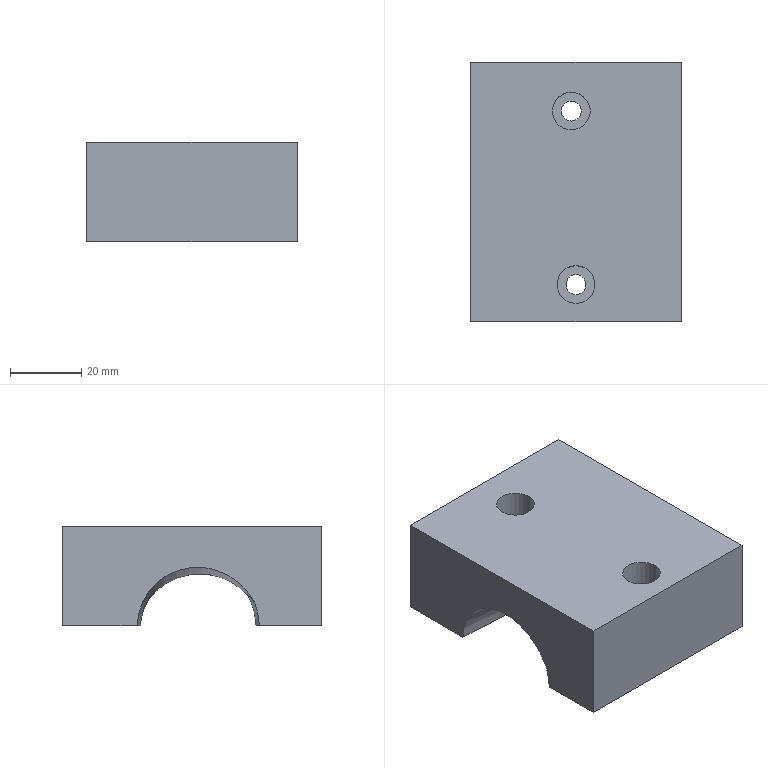NC program | NX | posted with a generic post | part box 59.014 x 72.744 x 27.972 mm
Lines 1 to 1690 of 94199, first 1532 of 1680 lines:
N10 G17 G21 G94 G90
(FLOOR_WALL_COPY_1 , TOOL : D63)
N12 T03 M6
N14 G54
N16 G17 G0 G90 X70.872 Y0. S6500 M3
N18 G43 Z30. H3
N20 Z10.025
N22 G94 G1 Z7.025 F1500.
N24 X67.872
N26 X-67.872
N28 X-70.872
N30 Z10.025
N32 G0 Z30.
N34 X70.872
N36 Z9.05
N38 G1 Z6.05
N40 X67.872
N42 X-67.872
N44 X-70.872
N46 Z9.05
N48 G0 Z30.
N50 X70.872
N52 Z8.075
N54 G1 Z5.075
N56 X67.872
N58 X-67.872
N60 X-70.872
N62 Z8.075
N64 G0 Z30.
N66 X70.872
N68 Z7.1
N70 G1 Z4.1
N72 X67.872
N74 X-67.872
N76 X-70.872
N78 Z7.1
N80 G0 Z30.
N82 X70.872
N84 Z6.125
N86 G1 Z3.125
N88 X67.872
N90 X-67.872
N92 X-70.872
N94 Z6.125
N96 G0 Z30.
N98 X70.872
N100 Z5.15
N102 G1 Z2.15
N104 X67.872
N106 X-67.872
N108 X-70.872
N110 Z5.15
N112 G0 Z30.
N114 X70.872
N116 Z4.175
N118 G1 Z1.175
N120 X67.872
N122 X-67.872
N124 X-70.872
N126 Z4.175
N128 G0 Z30.
N130 X70.872
N132 Z3.2
N134 G1 Z0.2
N136 X67.872
N138 X-67.872
N140 X-70.872
N142 Z3.2
N144 G0 Z30.
(FLOOR_WALL_COPY , TOOL : D63)
N146 X70.872
N148 Z3.
N150 G1 Z0.
N152 X67.872
N154 X-67.872
N156 X-70.872
N158 Z3.
N160 G0 Z30.
N162 M5
(ZLEVEL_PROFILE , TOOL : D10)
N164 T04 M6
N166 G54
N168 G17 G0 G90 X10.244 Y-35.541 S9500 M3
N170 G43 Z30. H4
N172 Z2.351
N174 G94 G1 Z-0.649 F1000.
N176 X12.69 Y-34.597
N178 G3 X13.318 Y-33.819 R1.
N180 G1 X13.332 Y-33.732 F3000.
N182 X14.234 Y-29.123
N184 X14.348 Y-28.585
N186 G3 X15.286 Y-19.404 R55.709
N188 X15.197 Y-18.502 R3.88
N190 G2 X13.462 Y5.443 R84.392
N192 G3 X13.42 Y6.979 R16.351
N194 G2 X13.599 Y29.292 R84.224
N196 X14.545 Y35.573 R362.838
N198 G1 X14.514 Y35.601 Z-1.296
N200 X14.477 Y35.4
N202 X13.767 Y30.791
N204 X13.538 Y29.165
N206 G3 X13.212 Y8.399 R83.745
N208 G1 X13.367 Y6.979
N210 G2 X13.409 Y5.443 R10.635
N212 G1 X13.319 Y3.906
N214 G3 X15.187 Y-18.634 R84.172
N216 G2 X15.254 Y-19.312 R2.871
N218 X14.202 Y-29.091 R56.887
N220 G1 X13.271 Y-33.837
N222 X13.192 Y-33.856 Z-1.939
N224 X14.151 Y-28.974
N226 G3 X15.176 Y-19.101 R54.964
N228 X15.131 Y-18.665 R1.888
N230 G2 X13.335 Y5.389 R83.356
N232 G3 X13.292 Y7.073 R8.768
N234 G2 X12.679 Y20.037 R87.094
N236 X13.595 Y30.023 R85.945
N238 G1 X14.407 Y35.4
N240 X14.453 Y35.633
N242 X14.376 Y35.669 Z-2.577
N244 X14.325 Y35.4
N246 X13.614 Y30.791
N248 X13.503 Y30.023
N250 G3 X13.162 Y7.448 R83.572
N252 G2 X13.221 Y5.23 R11.833
N254 G3 X14.985 Y-18.431 R83.939
N256 G2 X15.081 Y-19.474 R4.204
N258 G1 X15.066 Y-19.906
N260 G2 X14.088 Y-28.822 R52.674
N262 G1 X13.094 Y-33.866
N264 X13.021 Y-33.87 Z-2.893
N266 X12.961 Y-33.873 Z-3.208
N268 X12.981 Y-33.732
N270 X13.937 Y-28.998
N272 G3 X14.969 Y-19.654 R52.682
N274 X14.945 Y-18.706 R10.436
N276 G2 X13.103 Y5.296 R82.541
N278 G3 X13.052 Y7.356 R10.887
N280 G2 X12.975 Y26.95 R84.718
N282 X14.252 Y35.611 R281.865
N284 G1 X14.116 Y35.519 Z-3.831
N286 X13.489 Y31.559
N288 G3 X12.681 Y25.414 R113.024
N290 X12.88 Y7.747 R82.659
N292 G2 X12.963 Y5.443 R12.695
N294 G1 X12.92 Y4.674
N296 G3 X14.798 Y-18.645 R82.137
N298 G2 X14.851 Y-19.161 R2.163
N300 X13.936 Y-28.355 R56.288
N302 G1 X13.76 Y-29.123
N304 X12.982 Y-32.964
N306 X12.817 Y-33.879
N308 X12.738 Y-33.875 Z-4.138
N310 X12.645 Y-33.87 Z-4.444
N312 X13.916 Y-27.587
N314 G3 X14.7 Y-19.181 R54.369
N316 X14.643 Y-18.64 R2.276
N318 G2 X12.613 Y1.602 R82.074
N320 G1 X12.766 Y4.674
N322 X12.804 Y5.243
N324 G3 X12.733 Y7.747 R12.341
N326 G2 X12.89 Y28.486 R80.701
N328 X13.945 Y35.437 R440.926
N330 G1 X13.639 Y35.3 Z-5.043
N332 G2 X13.058 Y30.791 R60.606
N334 G1 X12.611 Y27.718
N336 X12.526 Y26.95
N338 G3 X12.557 Y7.747 R81.878
N340 G2 X12.633 Y5.443 R13.099
N342 G1 X12.577 Y4.674
N344 G3 X14.438 Y-18.464 R80.595
N346 G2 X14.522 Y-19.342 R3.428
N348 G1 X14.503 Y-19.906
N350 G2 X13.428 Y-29.123 R47.968
N352 G1 X13.268 Y-29.891
N354 X12.462 Y-33.858
N356 X12.356 Y-33.85 Z-5.334
N358 X12.255 Y-33.843 Z-5.624
N360 X12.436 Y-32.964
N362 X13.307 Y-28.768
N364 G3 X14.348 Y-18.823 R49.962
N366 G2 X12.436 Y5.443 R79.079
N368 G3 X12.379 Y7.747 R12.329
N370 G2 X12.653 Y29.255 R79.978
N372 G1 X12.804 Y30.213
N374 G3 X13.315 Y35.262 R56.984
N376 G1 X13.156 Y35.269 Z-5.908
N378 X12.997 Y35.276 Z-6.193
N380 G2 X12.572 Y30.023 R134.005
N382 G3 X12.175 Y7.747 R80.176
N384 G2 X12.216 Y5.443 R10.851
N386 G3 X13.867 Y-17.601 R78.874
N388 G1 X14.077 Y-18.541
N390 G2 X14.133 Y-19.113 R2.338
N392 G1 X14.112 Y-19.906
N394 G2 X13.192 Y-28.355 R48.034
N396 G1 X13.019 Y-29.123
N398 X12.034 Y-33.824
N400 X11.916 Y-33.817 Z-6.473
N402 X11.785 Y-33.81 Z-6.754
N404 X12.804 Y-29.067
N406 G3 X13.907 Y-18.725 R47.797
N408 G2 X11.831 Y3.138 R79.078
N410 G1 X11.992 Y5.443
N412 G3 X11.967 Y7.747 R11.595
N414 G2 X12.241 Y29.225 R78.57
N416 G3 X12.348 Y30.277 R10.864
N418 G1 X12.415 Y31.559
N420 X12.683 Y35.289
N422 X12.529 Y35.295 Z-7.026
N424 X12.378 Y35.302 Z-7.298
N426 X11.899 Y28.486
N428 G3 X11.3 Y12.356 R79.402
N430 G2 X11.737 Y6.445 R297.99
N432 X11.712 Y4.878 R9.86
N434 G1 X11.619 Y3.906
N436 G3 X13.688 Y-18.749 R78.587
N438 G2 X12.804 Y-27.88 R49.81
N440 G3 X11.519 Y-33.792 R606.821
N442 G1 X11.381 Y-33.782 Z-7.56
N444 X11.244 Y-33.772 Z-7.821
N446 X11.41 Y-32.964
N448 X12.379 Y-28.643
N450 G3 X13.352 Y-21.174 R41.302
N452 G1 X13.447 Y-18.69
N454 G2 X11.377 Y3.906 R77.127
N456 G1 X11.422 Y4.436
N458 G3 X11.43 Y5.461 R6.681
N460 G2 X10.943 Y14.881 R273.148
N462 X11.457 Y26.95 R78.516
N464 G1 X12.089 Y35.314
N466 X11.944 Y35.329 Z-8.073
N468 X11.782 Y35.346 Z-8.324
N470 X11.054 Y26.182
N472 G3 X10.725 Y10.051 R124.668
N474 G1 X10.763 Y9.283
N476 X11.129 Y3.906
N478 G3 X10.98 Y-1.471 R74.898
N480 X12.948 Y-17.601 R78.619
N482 G1 X13.123 Y-18.369
N484 X13.163 Y-18.722
N486 X13.146 Y-19.138
N488 G2 X12.165 Y-28.355 R43.893
N490 G1 X10.936 Y-33.75
N492 X10.797 Y-33.74 Z-8.568
N494 X10.64 Y-33.728 Z-8.811
N496 X12.032 Y-27.679
N498 G3 X12.891 Y-18.369 R46.52
N500 G2 X10.715 Y-1.471 R76.841
N502 X10.813 Y3.138 R82.834
N504 X10.669 Y26.182 R122.396
N506 G1 X11.485 Y35.381
N508 X11.343 Y35.398 Z-9.045
N510 X11.183 Y35.416 Z-9.28
N512 X10.273 Y26.182
N514 X10.091 Y23.878
N516 G3 X10.495 Y2.37 R109.189
N518 X10.461 Y0.272 R151.602
N520 X12.548 Y-17.983 R74.643
N522 G1 X12.604 Y-18.369
N524 X12.588 Y-19.138
N526 G2 X11.55 Y-28.419 R39.567
N528 G1 X10.316 Y-33.701
N530 X10.158 Y-33.687 Z-9.505
N532 X9.985 Y-33.671 Z-9.73
N534 X11.245 Y-28.485
N536 G3 X12.228 Y-21.088 R35.213
N538 G1 X12.308 Y-18.011
N540 G2 X10.189 Y0.408 R73.141
N542 G3 X10.105 Y1.844 R10.172
N544 G2 X9.604 Y22.746 R99.677
N546 G1 X9.883 Y26.182
N548 X10.858 Y35.453
N550 X10.708 Y35.47 Z-9.946
N552 X10.545 Y35.489 Z-10.162
N554 X9.422 Y25.517
N556 G3 X9.477 Y3.341 R96.947
N558 X9.896 Y0.066 R161.578
N560 X11.963 Y-17.601 R73.39
N562 G2 X11.996 Y-19.138 R6.001
N564 X10.91 Y-28.55 R37.741
N566 G1 X9.659 Y-33.641
N568 X9.491 Y-33.624 Z-10.368
N570 X9.311 Y-33.605 Z-10.574
N572 G3 X11.134 Y-26.051 R120.535
N574 X11.69 Y-17.601 R44.58
N576 G2 X9.642 Y-1.548 R74.685
N578 G3 X9.57 Y-0.692 R6.581
N580 G1 X9.226 Y1.602
N582 G2 X8.844 Y23.878 R87.033
N584 G1 X9.083 Y26.182
N586 X10.21 Y35.526
N588 X10.053 Y35.544 Z-10.77
N590 X9.883 Y35.563 Z-10.967
N592 X8.605 Y25.669
N594 G3 X7.81 Y11.588 R97.875
N596 X9.369 Y-2.239 R99.053
N598 X11.367 Y-17.248 R75.126
N600 G2 X10.489 Y-27.731 R40.2
N602 G1 X8.978 Y-33.569
N604 X8.812 Y-33.552 Z-11.153
N606 X8.618 Y-33.531 Z-11.339
N608 X10.192 Y-27.587
N610 X10.37 Y-26.819
N612 G3 X11.031 Y-16.833 R40.131
N614 G2 X9.168 Y-3.775 R73.819
N616 X8.033 Y3.138 R985.26
N618 X7.859 Y23.11 R75.535
N620 X9.553 Y35.6 R1001.089
N622 G1 X9.386 Y35.618 Z-11.515
N624 X9.221 Y35.637 Z-11.691
N626 X7.713 Y25.414
N628 X7.243 Y21.624
N630 G3 X7.41 Y3.969 R66.674
N632 X8.945 Y-4.75 R138.157
N634 X10.616 Y-16.065 R80.897
N636 G2 X9.717 Y-28.269 R35.231
N638 G1 X8.271 Y-33.492
N640 X8.094 Y-33.472 Z-11.857
N642 X7.911 Y-33.45 Z-12.022
N644 X8.051 Y-32.964
N646 X9.717 Y-26.986
N648 G3 X10.21 Y-15.297 R35.008
N650 G2 X8.783 Y-6.079 R90.765
N652 G1 X7.545 Y0.066
N654 X7.265 Y1.537
N656 G2 X6.648 Y20.47 R61.369
N658 G1 X7.067 Y23.878
N660 X8.901 Y35.672
N662 X8.729 Y35.692 Z-12.177
N664 X8.566 Y35.71 Z-12.332
N666 X6.502 Y23.11
N668 X6.143 Y20.353
N670 G3 X5.885 Y6.979 R60.76
N672 X8.557 Y-6.848 R140.299
N674 X9.949 Y-15.297 R169.214
N676 G2 X9.44 Y-26.819 R36.947
N678 G1 X9.249 Y-27.587
N680 X7.564 Y-33.408
N682 X7.391 Y-33.385 Z-12.477
N684 X7.221 Y-33.362 Z-12.622
N686 X7.401 Y-32.789
N688 X8.945 Y-27.627
N690 X9.141 Y-26.819
N692 G3 X9.42 Y-13.761 R35.75
N694 G1 X9.272 Y-12.993
N696 X9.144 Y-12.224
N698 G3 X6.773 Y-1.013 R134.514
N700 G2 X5.584 Y19.772 R54.025
N702 G1 X6.043 Y23.11
N704 X8.25 Y35.746
N706 X8.091 Y35.765 Z-12.756
N708 X7.934 Y35.784 Z-12.889
N710 X5.599 Y23.11
N712 X5.259 Y20.805
N714 X4.933 Y18.628
N716 G3 X5.416 Y2.983 R43.75
N718 G1 X6.204 Y-0.702
N720 G2 X9.227 Y-14.529 R118.409
N722 X8.854 Y-26.819 R34.94
N724 G1 X8.648 Y-27.587
N726 X6.885 Y-33.313
N728 X6.728 Y-33.289 Z-13.012
N730 X6.566 Y-33.264 Z-13.134
N732 X8.365 Y-27.587
N734 X8.568 Y-26.819
N736 G3 X8.945 Y-14.695 R32.979
N738 X6.132 Y-2.239 R98.202
N740 G2 X3.925 Y9.283 R55.566
N742 X4.729 Y20.551 R50.892
N744 G1 X5.085 Y22.483
N746 X5.178 Y23.11
N748 X7.638 Y35.821
N750 X7.501 Y35.838 Z-13.246
N752 X7.363 Y35.855 Z-13.358
N754 X4.313 Y20.873
N756 X4.151 Y20.037
N758 G3 X3.896 Y4.674 R42.458
N760 G1 X4.234 Y3.138
N762 X7.18 Y-7.665
N764 G2 X8.969 Y-17.421 R58.43
N766 X7.859 Y-28.355 R28.007
N768 G1 X6.252 Y-33.209
N770 X6.108 Y-33.184 Z-13.458
N772 X5.965 Y-33.159 Z-13.558
N774 X7.84 Y-27.587
N776 X8.061 Y-26.819
N778 G3 X8.463 Y-15.297 R29.811
N780 X5.469 Y-3.007 R77.185
N782 G1 X4.962 Y-1.471
N784 G2 X2.755 Y8.515 R55.165
N786 X3.459 Y18.844 R39.058
N788 G1 X3.858 Y20.805
N790 X6.629 Y33.506
N792 X7.097 Y35.891
N794 G3 X6.773 Y36.837 R1.
N796 G1 X4.848 Y38.516
N798 Z-10.558
N800 G0 Z30.
N802 X-7.808 Y37.382
N804 Z2.351
N806 G1 Z-0.649 F1000.
N808 X-9.983 Y35.98
N810 G3 X-10.44 Y35.091 R1.
N812 G2 X-10.193 Y29.255 R446.101 F3000.
N814 G1 X-9.511 Y16.964
N816 X-9.407 Y14.793
N818 G2 X-9.866 Y-3.186 R122.787
N820 G1 X-10.762 Y-12.224
N822 G3 X-11.187 Y-19.963 R97.835
N824 X-10.376 Y-29.019 R43.623
N826 G1 X-9.436 Y-33.815
N828 X-9.387 Y-33.83 Z-1.296
N830 X-9.544 Y-32.964
N832 X-10.302 Y-29.123
N834 X-10.353 Y-28.92
N836 G2 X-11.028 Y-23.746 R39.014
N838 G1 X-11.057 Y-22.978
N840 X-11.124 Y-22.21
N842 G2 X-11.124 Y-18.453 R110.474
N844 G3 X-11.013 Y-16.065 R46.666
N846 G2 X-10.359 Y-8.611 R202.692
N848 G3 X-9.645 Y-1.471 R585.412
N850 X-9.205 Y8.515 R113.819
N852 X-9.378 Y15.428 R152.84
N854 X-9.987 Y26.182 R461.108
N856 G1 X-10.37 Y34.631
N858 X-10.396 Y35.144
N860 X-10.335 Y35.186 Z-1.939
N862 X-10.3 Y34.631
N864 X-9.981 Y27.718
N866 X-9.938 Y26.95
N868 X-9.35 Y16.964
N870 X-9.244 Y14.66
N872 G2 X-9.699 Y-3.007 R118.11
N874 G1 X-9.847 Y-4.543
N876 X-10.49 Y-10.688
N878 G3 X-11.07 Y-20.674 R99.491
N880 X-10.53 Y-27.587 R47.233
N882 G1 X-10.393 Y-28.355
N884 X-9.314 Y-33.847
N886 X-9.208 Y-33.857 Z-2.577
N888 X-10.256 Y-28.514
N890 G2 X-10.905 Y-23.146 R36.873
N892 X-10.734 Y-14.529 R64.491
N894 X-9.742 Y-4.543 R359.94
N896 G3 X-9.043 Y4.674 R146.008
N898 X-9.076 Y13.327 R130.573
N900 X-9.504 Y21.563 R276.789
N902 G2 X-10.24 Y35.195 R530.755
N904 G1 X-10.185 Y35.199 Z-2.893
N906 X-10.139 Y35.203 Z-3.208
N908 G3 X-9.666 Y26.182 R1124.487
N910 G1 X-9.516 Y23.878
N912 X-9.465 Y23.11
N914 G2 X-9.04 Y16.139 R568.997
N916 X-8.909 Y3.906 R139.195
N918 X-9.842 Y-6.848 R174.936
N920 G3 X-10.675 Y-15.363 R223.861
N922 X-10.765 Y-23.746 R62.101
N924 X-10.029 Y-29.123 R37.612
N926 G1 X-9.867 Y-29.891
N928 X-9.086 Y-33.863
N930 X-9.008 Y-33.864 Z-3.52
N932 X-8.934 Y-33.866 Z-3.831
N934 X-9.889 Y-29.123
N936 X-10.051 Y-28.355
N938 G2 X-10.662 Y-17.601 R45.697
N940 X-9.935 Y-9.152 R127.722
N942 G3 X-9.053 Y-0.702 R291.588
N944 X-8.667 Y11.588 R104.753
N946 G1 X-8.99 Y18.501
N948 G2 X-9.996 Y35.215 R769.386
N950 G1 X-9.91 Y35.221 Z-4.138
N952 X-9.822 Y35.227 Z-4.444
N954 G3 X-9.186 Y23.878 R640.786
N956 G1 X-9.056 Y22.341
N958 X-8.996 Y21.573
N960 X-8.966 Y20.805
N962 G2 X-8.516 Y13.124 R231.159
N964 X-8.986 Y-2.239 R105.26
N966 X-9.932 Y-10.688 R781.442
N968 G3 X-10.565 Y-18.951 R114.064
N970 X-9.756 Y-29.016 R42.1
N972 G1 X-8.798 Y-33.732
N974 X-8.777 Y-33.867
N976 X-8.678 Y-33.862 Z-4.744
N978 X-8.583 Y-33.857 Z-5.043
N980 X-9.581 Y-29.031
N982 G2 X-10.388 Y-19.222 R41.455
N984 X-9.75 Y-10.879 R106.308
N986 G1 X-8.925 Y-3.775
N988 X-8.764 Y-2.239
N990 G3 X-8.225 Y11.588 R99.983
N992 X-8.731 Y20.805 R225.203
N994 G2 X-9.644 Y35.24 R426.911
N996 G1 X-9.553 Y35.246 Z-5.334
N998 X-9.447 Y35.252 Z-5.624
N1000 G3 X-8.809 Y24.739 R449.887
N1002 G1 X-8.665 Y23.11
N1004 X-8.268 Y17.548
N1006 G2 X-7.92 Y8.324 R136.877
N1008 X-8.282 Y0.222 R83.479
N1010 G1 X-8.512 Y-2.239
N1012 X-8.579 Y-3.007
N1014 X-8.674 Y-3.775
N1016 X-8.776 Y-4.543
N1018 X-9.684 Y-12.224
N1020 X-9.894 Y-14.461
N1022 G3 X-10.21 Y-20.861 R72.663
N1024 X-9.41 Y-28.89 R38.624
N1026 G1 X-8.385 Y-33.846
N1028 X-8.262 Y-33.837 Z-5.908
N1030 X-8.15 Y-33.829 Z-6.193
N1032 X-9.305 Y-28.355
N1034 G2 X-9.958 Y-18.369 R40.916
N1036 X-8.891 Y-7.616 R141.923
N1038 G3 X-8.306 Y-3.007 R212.591
N1040 G1 X-8.238 Y-2.239
N1042 X-8.065 Y-0.702
N1044 X-7.914 Y1.064
N1046 G3 X-7.681 Y12.195 R86.708
N1048 G1 X-7.755 Y13.892
N1050 G3 X-8.353 Y22.341 R271.693
N1052 G2 X-9.241 Y35.264 R406.061
N1054 G1 X-9.121 Y35.271 Z-6.473
N1056 X-9.003 Y35.278 Z-6.754
N1058 G3 X-8.001 Y21.573 R369.34
N1060 G1 X-7.933 Y20.805
N1062 X-7.596 Y16.32
N1064 G2 X-7.43 Y3.138 R105.532
N1066 G1 X-7.759 Y-0.702
N1068 G2 X-8.908 Y-9.92 R320.186
N1070 G3 X-9.756 Y-19.405 R101.404
N1072 X-8.947 Y-28.933 R37.787
N1074 G1 X-7.9 Y-33.812
N1076 X-7.77 Y-33.804 Z-7.026
N1078 X-7.638 Y-33.796 Z-7.298
N1080 X-7.796 Y-32.964
N1082 X-8.686 Y-28.978
N1084 G2 X-9.531 Y-20.649 R35.322
N1086 X-8.856 Y-11.678 R78.251
N1088 G1 X-7.595 Y-2.239
N1090 X-7.52 Y-1.471
N1092 X-7.423 Y-0.702
N1094 G3 X-7.107 Y13.892 R86.944
N1096 X-8.037 Y25.194 R275.313
N1098 G1 X-8.421 Y30.023
N1100 G3 X-8.753 Y35.293 R145.709
N1102 G1 X-8.623 Y35.302 Z-7.56
N1104 X-8.477 Y35.311 Z-7.821
N1106 G3 X-7.368 Y21.573 R313.598
N1108 G2 X-6.633 Y11.438 R148.06
N1110 X-7.282 Y-2.359 R81.406
N1112 X-8.475 Y-11.072 R1051.255
N1114 G3 X-9.215 Y-18.439 R92.262
N1116 X-8.809 Y-27.086 R40.563
N1118 X-7.357 Y-33.775 R1700.526
N1120 G1 X-7.208 Y-33.763 Z-8.073
N1122 X-7.057 Y-33.751 Z-8.324
N1124 X-8.105 Y-29.123
N1126 G2 X-8.872 Y-24.514 R35.129
N1128 X-8.672 Y-15.297 R47.716
N1130 X-7.235 Y-4.693 R225.714
N1132 G3 X-6.326 Y13.195 R83.374
N1134 X-7.055 Y21.977 R169.123
N1136 G2 X-8.205 Y35.329 R290.272
N1138 G1 X-8.077 Y35.338 Z-8.568
N1140 X-7.925 Y35.348 Z-8.811
N1142 X-7.25 Y26.95
N1144 G2 X-6.015 Y14.66 R310.631
N1146 X-6.631 Y-3.007 R77.1
N1148 X-7.796 Y-10.719 R2179.035
N1150 G3 X-8.69 Y-19.311 R90.208
N1152 X-7.85 Y-29.019 R34.378
N1154 G1 X-6.755 Y-33.726
N1156 X-6.598 Y-33.712 Z-9.045
N1158 X-6.438 Y-33.698 Z-9.28
N1160 X-7.697 Y-28.355
N1162 G2 X-8.434 Y-20.865 R30.899
N1164 X-7.716 Y-12.459 R68.938
N1166 G1 X-7.341 Y-9.92
N1168 X-6.351 Y-3.775
N1170 X-6.125 Y-2.239
N1172 G3 X-5.388 Y11.588 R76.769
N1174 X-6.409 Y22.689 R193.116
N1176 G2 X-7.62 Y35.37 R250.441
N1178 G1 X-7.489 Y35.38 Z-9.505
N1180 X-7.326 Y35.391 Z-9.73
N1182 X-7.266 Y34.631
N1184 X-6.548 Y26.95
N1186 X-5.71 Y19.967
N1188 G2 X-5.135 Y14.438 R175.423
N1190 X-5.654 Y-1.793 R67.999
N1192 X-6.983 Y-9.92 R396.157
N1194 G3 X-8.094 Y-19.138 R82.702
N1196 X-7.212 Y-29.123 R32.402
N1198 G1 X-7.022 Y-29.891
N1200 X-6.104 Y-33.665
N1202 X-5.962 Y-33.651 Z-9.946
N1204 X-5.784 Y-33.634 Z-10.162
N1206 X-7.266 Y-27.587
N1208 G2 X-7.731 Y-18.369 R33.33
N1210 X-6.357 Y-8.384 R89.029
N1212 G3 X-4.501 Y4.674 R113.083
N1214 X-5.192 Y19.269 R81.307
N1216 G2 X-7.01 Y35.415 R295.073
N1218 G1 X-6.862 Y35.427 Z-10.368
N1220 X-6.694 Y35.44 Z-10.574
N1222 G3 X-4.561 Y17.733 R329.111
N1224 G2 X-4.142 Y3.138 R68.234
N1226 X-5.972 Y-8.384 R129.415
N1228 G3 X-7.431 Y-18.369 R89.492
N1230 X-6.493 Y-29.503 R31.685
N1232 G1 X-5.432 Y-33.602
N1234 X-5.263 Y-33.586 Z-10.77
N1236 X-5.085 Y-33.571 Z-10.967
N1238 X-6.277 Y-29.034
N1240 G2 X-7.083 Y-17.889 R30.423
N1242 X-5.126 Y-6.079 R115.645
N1244 G3 X-3.484 Y5.443 R84.483
N1246 X-4.3 Y19.269 R73.
N1248 G2 X-6.378 Y35.465 R249.012
N1250 G1 X-6.222 Y35.478 Z-11.153
N1252 X-6.051 Y35.493 Z-11.339
N1254 G3 X-3.966 Y19.998 R236.49
N1256 G2 X-2.878 Y7.747 R78.74
N1258 X-4.517 Y-5.114 R69.218
N1260 G3 X-6.551 Y-16.065 R150.783
N1262 X-6.482 Y-26.819 R34.194
N1264 G1 X-6.31 Y-27.587
N1266 X-4.73 Y-33.535
N1268 X-4.557 Y-33.516 Z-11.515
N1270 X-4.378 Y-33.496 Z-11.691
N1272 X-5.81 Y-28.355
N1274 G2 X-6.42 Y-17.601 R29.376
N1276 X-4.126 Y-5.311 R120.054
N1278 G3 X-2.347 Y7.747 R63.655
N1280 X-3.511 Y20.037 R70.245
N1282 G2 X-5.74 Y35.52 R236.179
N1284 G1 X-5.575 Y35.535 Z-11.857
N1286 X-5.408 Y35.551 Z-12.022
N1288 G3 X-2.775 Y18.501 R235.49
N1290 G2 X-3.406 Y-4.04 R52.249
N1292 G3 X-5.902 Y-16.065 R165.767
N1294 X-5.854 Y-26.819 R31.71
N1296 G1 X-5.721 Y-27.442
N1298 X-4.029 Y-33.455
N1300 X-3.856 Y-33.432 Z-12.177
N1302 X-3.679 Y-33.409 Z-12.332
N1304 X-4.996 Y-28.933
N1306 G2 X-5.873 Y-18.367 R26.25
N1308 X-3.632 Y-6.848 R82.071
N1310 G3 X-1.338 Y5.443 R77.728
N1312 X-2.278 Y18.501 R51.939
N1314 G2 X-5.095 Y35.581 R216.921
N1316 G1 X-4.94 Y35.597 Z-12.477
N1318 X-4.784 Y35.612 Z-12.622
N1320 G3 X-1.929 Y19.269 R178.983
N1322 G2 X-1.396 Y0.834 R45.853
N1324 G1 X-1.712 Y-0.702
N1326 X-4.177 Y-10.65
N1328 G3 X-5.713 Y-20.154 R53.751
N1330 X-4.766 Y-28.637 R23.626
N1332 G1 X-3.341 Y-33.363
N1334 X-3.173 Y-33.338 Z-12.756
N1336 X-3.002 Y-33.312 Z-12.889
N1338 X-4.361 Y-28.986
N1340 G2 X-5.303 Y-18.596 R24.564
N1342 X-3.026 Y-7.616 R69.397
N1344 G3 X-0.48 Y3.138 R99.8
N1346 X-1.432 Y19.269 R45.088
N1348 G2 X-4.48 Y35.644 R160.733
N1350 G1 X-4.337 Y35.66 Z-13.012
N1352 X-4.198 Y35.675 Z-13.134
N1354 G3 X-0.948 Y19.269 R151.009
N1356 G1 X-0.303 Y16.258
N1358 G2 X-0.899 Y-1.387 R36.391
N1360 G3 X-3.869 Y-12.224 R491.006
N1362 X-5.2 Y-21.845 R40.823
N1364 X-4.228 Y-28.452 R20.407
N1366 G1 X-2.685 Y-33.262
N1368 X-2.535 Y-33.235 Z-13.246
N1370 X-2.381 Y-33.207 Z-13.358
N1372 X-2.634 Y-32.471
N1374 X-3.966 Y-28.388
N1376 G2 X-4.938 Y-21.093 R20.243
N1378 X-3.276 Y-11.155 R43.739
N1380 G1 X-0.158 Y-0.357
N1382 G3 X0.406 Y15.18 R32.067
N1384 G1 X-0.459 Y19.269
N1386 G2 X-3.918 Y35.708 R132.758
N1388 G1 X-3.789 Y35.723 Z-13.458
N1390 X-3.659 Y35.739 Z-13.558
N1392 G3 X-0.171 Y20.037 R108.953
N1394 G2 X1.717 Y7.747 R44.161
N1396 X-0.847 Y-4.274 R46.086
N1398 G3 X-4.385 Y-17.601 R81.85
N1400 X-3.406 Y-29.324 R23.181
N1402 G1 X-3.21 Y-29.891
N1404 X-2.097 Y-33.152
N1406 X-1.971 Y-33.128 Z-13.648
N1408 X-1.835 Y-33.101 Z-13.739
N1410 X-3.719 Y-27.587
N1412 X-3.935 Y-26.819
N1414 G2 X-3.887 Y-16.065 R25.126
N1416 X-0.049 Y-3.033 R99.301
N1418 G3 X2.299 Y7.367 R40.248
N1420 X4.539 Y-1.471 R45.918
N1422 G2 X7.82 Y-12.993 R89.022
N1424 X8.182 Y-25.283 R32.816
N1426 X5.693 Y-33.106 R59.891
N1428 G1 X5.555 Y-33.077 Z-13.826
N1430 X5.414 Y-33.047 Z-13.914
N1432 G3 X7.95 Y-25.283 R51.28
N1434 X7.84 Y-14.507 R30.262
N1436 X4.313 Y-2.097 R73.482
N1438 G1 X4.068 Y-1.471
N1440 X2.546 Y3.138
N1442 X2.394 Y3.701
N1444 G2 X-0.693 Y-6.079 R83.994
N1446 G3 X-4.102 Y-18.995 R57.289
N1448 X-3.153 Y-28.569 R20.239
N1450 G1 X-1.862 Y-32.234
N1452 X-1.545 Y-33.042
N1454 X-1.398 Y-33.012 Z-14.001
N1456 X-1.252 Y-32.982 Z-14.088
N1458 X-2.71 Y-29.123
N1460 G2 X-3.953 Y-19.906 R19.59
N1462 X-1.177 Y-8.384 R47.734
N1464 G1 X2.453 Y1.4
N1466 X2.77 Y0.732
N1468 X3.826 Y-2.239
N1470 X4.163 Y-3.007
N1472 G2 X7.838 Y-16.065 R60.096
N1474 X7.361 Y-26.819 R26.457
N1476 G1 X7.122 Y-27.587
N1478 X5.134 Y-32.988
N1480 X4.99 Y-32.951 Z-14.176
N1482 X4.835 Y-32.911 Z-14.263
N1484 G3 X7.485 Y-25.283 R50.071
N1486 X6.993 Y-12.993 R29.609
N1488 X2.521 Y-0.367 R71.88
N1490 X-2.122 Y-12.224 R115.606
N1492 X-3.791 Y-22.613 R32.458
N1494 X-2.647 Y-28.611 R16.585
N1496 G1 X-1.09 Y-32.582
N1498 X-0.946 Y-32.91
N1500 X-0.794 Y-32.872 Z-14.35
N1502 X-0.631 Y-32.831 Z-14.437
N1504 X-2.634 Y-27.854
N1506 G2 X-3.158 Y-17.601 R20.047
N1508 X2.514 Y-1.979 R57.99
N1510 X7.377 Y-16.471 R47.314
N1512 X6.629 Y-27.529 R24.403
N1514 G1 X4.529 Y-32.829
N1516 X4.374 Y-32.785 Z-14.526
N1518 X4.201 Y-32.736 Z-14.615
N1520 X4.313 Y-32.498
N1522 X6.317 Y-27.587
N1524 G3 X7.297 Y-18.079 R22.244
N1526 X2.503 Y-3.347 R38.847
N1528 X-2.882 Y-17.601 R48.23
N1530 X-2.634 Y-27.012 R20.112
N1532 G1 X-2.439 Y-27.587
N1534 X-0.306 Y-32.748
N1536 X-0.138 Y-32.693 Z-14.702
N1538 X0.039 Y-32.636 Z-14.789
N1540 X-1.525 Y-29.123
N1542 G2 X-2.848 Y-19.138 R17.308
N1544 X2.494 Y-4.586 R40.044
N1546 X6.221 Y-13.761 R31.888
N1548 G1 X6.514 Y-15.013
N1550 G2 X6.708 Y-25.283 R24.564
N1552 X3.848 Y-32.629 R38.735
N1554 G1 X3.665 Y-32.569 Z-14.877
N1556 X3.483 Y-32.509 Z-14.966
N1558 G3 X6.707 Y-23.746 R28.391
N1560 X2.501 Y-5.839 R28.375
N1562 X-2.664 Y-19.906 R33.507
N1564 X-1.196 Y-29.123 R16.317
N1566 G1 X0.403 Y-32.514
N1568 X0.593 Y-32.435 Z-15.053
N1570 X0.786 Y-32.354 Z-15.14
N1572 X0.454 Y-31.762
N1574 X-0.834 Y-29.123
N1576 X-1.09 Y-28.58
N1578 G2 X-2.486 Y-21.442 R14.637
N1580 X2.494 Y-6.998 R28.651
N1582 X6.42 Y-23.746 R25.722
N1584 X3.096 Y-32.348 R24.995
N1586 G1 X2.891 Y-32.256 Z-15.229
N1588 X2.684 Y-32.163 Z-15.317
N1590 G3 X5.857 Y-25.147 R26.476
N1592 X2.479 Y-8.051 R23.367
N1594 X-2.187 Y-21.497 R26.173
N1596 X-0.921 Y-28.117 R13.751
N1598 G1 X-0.452 Y-29.123
N1600 X1.196 Y-32.175
N1602 X1.19 Y-31.873 Z-15.376
N1604 X1.187 Y-31.569 Z-15.435
N1606 X1.196 Y-31.258 Z-15.493
N1608 X0.454 Y-30.063
N1610 G2 X-1.902 Y-22.21 R14.837
N1612 X2.471 Y-9.107 R23.636
N1614 X5.815 Y-23.746 R22.089
N1616 X2.265 Y-31.909 R20.488
N1618 G1 X1.998 Y-32.35
N1620 X1.93 Y-32.458
N1622 X1.606 Y-31.916
N1624 X1.196 Y-31.258
N1626 G2 X1.164 Y-30.258 R1.
N1628 G1 X1.923 Y-26.384
N1630 Z-12.493
N1632 G0 Z30.
N1634 X2.658 Y-21.56
N1636 Z-12.671
N1638 G1 Z-15.671 F1000.
N1640 X5.119 Y-19.677
N1642 G3 X5.503 Y-18.754 R1.
N1644 G1 X5.453 Y-18.369 F3000.
N1646 G3 X2.455 Y-10.191 R19.567
N1648 X-1.497 Y-23.746 R20.774
N1650 X1.923 Y-31.464 R16.111
N1652 X5.553 Y-19.138 R16.316
N1654 G1 X5.503 Y-18.754
N1656 X5.337 Y-18.774 Z-15.76
N1658 X5.155 Y-18.796 Z-15.849
N1660 G2 X5.223 Y-19.46 R17.813
N1662 G1 X5.261 Y-19.906
N1664 G2 X1.922 Y-30.575 R14.357
N1666 X-1.16 Y-23.746 R14.056
N1668 X2.429 Y-11.275 R18.829
N1670 X5.155 Y-18.796 R17.813
N1672 G1 X4.964 Y-18.822 Z-15.939
N1674 X4.771 Y-18.848 Z-16.029
N1676 G3 X2.398 Y-12.378 R16.077
N1678 X-0.782 Y-23.746 R16.956
N1680 X1.92 Y-29.671 R11.576
N1682 X4.936 Y-20.674 R12.498
N1684 G1 X4.88 Y-19.906
N1686 G3 X4.771 Y-18.848 R16.077
N1688 G1 X4.566 Y-18.881 Z-16.118
N1690 X4.37 Y-18.912 Z-16.207
N1692 G2 X4.554 Y-21.442 R15.052
N1694 G1 X4.546 Y-22.21
N1696 G2 X1.919 Y-28.783 R10.392
N1698 X-0.425 Y-23.451 R8.655
N1700 X2.371 Y-13.458 R15.391
N1702 X4.37 Y-18.912 R15.052
N1704 G1 X4.153 Y-18.95 Z-16.295
N1706 X3.938 Y-18.989 Z-16.383
N1708 G3 X2.34 Y-14.586 R13.702
N1710 X0.164 Y-24.454 R13.225
N1712 X1.919 Y-27.904 R6.641
N1714 X4.144 Y-22.21 R8.825
N1716 G1 X4.15 Y-21.442
N1718 G3 X3.938 Y-18.989 R13.702
N1720 G1 X3.942 Y-19.344 Z-16.405
N1722 X3.931 Y-19.698 Z-16.428
N1724 X3.91 Y-20.053 Z-16.45
N1726 X3.888 Y-20.408 Z-16.472
N1728 X3.86 Y-20.763 Z-16.494
N1730 X3.811 Y-21.117 Z-16.517
N1732 X3.748 Y-21.471 Z-16.539
N1734 X3.706 Y-21.826 Z-16.561
N1736 X3.703 Y-22.21
N1738 G2 X1.92 Y-27.023 R7.684
N1740 X0.638 Y-24.514 R5.661
N1742 X2.298 Y-15.842 R11.319
N1744 X3.709 Y-21.442 R11.492
N1746 G1 X3.706 Y-21.826
N1748 X3.464 Y-21.814 Z-16.65
N1750 X3.27 Y-21.805 Z-16.739
N1752 G3 X2.226 Y-17.126 R9.07
N1754 X0.966 Y-23.746 R10.33
N1756 X1.93 Y-26.134 R5.526
N1758 X3.27 Y-21.805 R9.07
N1760 X2.812 Y-20.916 R1.
N1762 G1 Z-13.739
N1764 G0 Z30.
N1766 X1.388 Y-21.818
N1768 Z-13.739
N1770 G1 Z-16.916 F1000.
N1772 G2 X2.168 Y-18.622 R8.088 F3000.
N1774 X1.946 Y-25.061 R8.187
N1776 X1.388 Y-21.818 R8.088
N1778 X1.918 Y-20.97 R1.
N1780 G1 Z-13.916
N1782 G0 Z30.
N1784 X-1.078 Y38.276
N1786 Z-10.739
N1788 G1 Z-13.739 F1000.
N1790 X-3.056 Y36.699
N1792 G3 X-3.422 Y35.768 R1.
N1794 X0.037 Y20.805 R98.822 F3000.
N1796 G2 X2.131 Y12.07 R65.416
N1798 X3.233 Y20.037 R43.918
N1800 G3 X6.856 Y35.924 R613.953
N1802 G1 X6.737 Y35.941 Z-13.826
N1804 X6.618 Y35.957 Z-13.914
N1806 X6.496 Y35.4
N1808 X5.085 Y29.144
N1810 X2.414 Y18.501
N1812 X1.927 Y16.196
N1814 X0.757 Y20.037
N1816 X0.454 Y20.841
N1818 G2 X-3.176 Y35.802 R94.803
N1820 G1 X-3.053 Y35.819 Z-14.001
N1822 X-2.925 Y35.836 Z-14.088
N1824 G3 X1.812 Y18.403 R92.007
N1826 X6.363 Y36. R353.162
N1828 G1 X6.24 Y36.021 Z-14.176
N1830 X6.103 Y36.044 Z-14.263
N1832 G2 X1.722 Y20.449 R160.798
N1834 X-2.671 Y35.872 R70.041
N1836 G1 X-2.538 Y35.893 Z-14.35
N1838 X-2.397 Y35.914 Z-14.437
N1840 G3 X1.659 Y22.064 R60.998
N1842 X5.842 Y36.089 R119.145
N1844 G1 X5.704 Y36.119 Z-14.526
N1846 X5.566 Y36.149 Z-14.615
N1848 G2 X1.602 Y23.652 R86.605
N1850 X-2.112 Y35.96 R52.963
N1852 G1 X-1.97 Y35.983 Z-14.702
N1854 X-1.826 Y36.006 Z-14.789
N1856 G3 X1.56 Y25.097 R48.753
N1858 X5.282 Y36.218 R69.247
N1860 G1 X5.133 Y36.253 Z-14.877
N1862 X4.979 Y36.29 Z-14.966
N1864 G2 X1.531 Y26.458 R58.005
N1866 X-1.505 Y36.067 R45.112
N1868 G1 X-1.35 Y36.097 Z-15.053
N1870 X-1.186 Y36.128 Z-15.14
N1872 G3 X1.509 Y27.802 R42.474
N1874 X4.659 Y36.355 R48.05
N1876 G1 X4.487 Y36.39 Z-15.229
N1878 X4.323 Y36.424 Z-15.317
N1880 G2 X1.513 Y29.123 R44.985
N1882 X-0.842 Y36.202 R41.687
N1884 G1 X-0.666 Y36.243 Z-15.405
N1886 X-0.487 Y36.284 Z-15.493
N1888 G3 X1.558 Y30.422 R35.88
N1890 G1 X1.998 Y31.302
N1892 X3.955 Y36.511
N1894 X3.769 Y36.556 Z-15.582
N1896 X3.562 Y36.606 Z-15.671
N1898 X1.564 Y31.718
N1900 X-0.105 Y36.384
N1902 X0.101 Y36.443 Z-15.76
N1904 X0.299 Y36.5 Z-15.849
N1906 X1.589 Y33.128
N1908 X2.925 Y36.168
N1910 X3.143 Y36.732
N1912 X2.93 Y36.798 Z-15.939
N1914 X2.703 Y36.869 Z-16.029
N1916 X1.696 Y34.631
N1918 X1.617 Y34.493
N1920 X0.747 Y36.654
N1922 X0.976 Y36.74 Z-16.118
N1924 X1.214 Y36.828 Z-16.207
N1926 X1.646 Y35.828
N1928 X2.247 Y37.046
N1930 G3 X2.181 Y38.044 R1.
N1932 G1 X-0.835 Y42.556
N1934 Z-13.207
N1936 G0 Z30.
N1938 M5
(ZLEVEL_PROFILE_COPY , TOOL : D6)
N1940 T16 M6
N1942 G54
N1944 G17 G0 G90 X2.76 Y5.194 S9500 M3
N1946 G43 Z30. H16
N1948 Z-10.768
N1950 G94 G1 Z-13.768 F1000.
N1952 X4.088 Y6.251
N1954 G3 X4.308 Y6.809 R0.6
N1956 G2 X4.031 Y12.583 R28.725 F2500.
N1958 G1 X4.022 Y12.857 Z-13.779
N1960 X4.017 Y13.131 Z-13.789
N1962 X4.013 Y13.405 Z-13.8
N1964 X4.01 Y13.679 Z-13.811
N1966 X4.008 Y13.953 Z-13.822
N1968 X4.005 Y14.227 Z-13.832
N1970 X3.993 Y14.502 Z-13.843
N1972 X3.976 Y14.778 Z-13.854
N1974 X3.985 Y15.05 Z-13.864
N1976 G3 X3.538 Y11.457 R69.805
N1978 X4.242 Y5.074 R28.323
N1980 G1 X4.252 Y4.805 Z-13.882
N1982 X4.271 Y4.539 Z-13.9
N1984 X4.295 Y4.275 Z-13.917
N1986 X4.308 Y4.007 Z-13.935
N1988 X4.309 Y3.736 Z-13.952
N1990 G2 X3.527 Y6.661 R61.828
N1992 X3.606 Y15.054 R22.622
N1994 X3.893 Y16.374 R239.988
N1996 G1 X3.853 Y16.664 Z-13.979
N1998 X3.836 Y16.95 Z-14.006
N2000 X3.793 Y17.241 Z-14.032
N2002 G3 X3.414 Y15.659 R332.344
N2004 X3.592 Y4.862 R21.885
N2006 G1 X4.406 Y2.581
N2008 X4.361 Y2.341 Z-14.056
N2010 X4.366 Y2.119 Z-14.08
N2012 X4.371 Y1.898 Z-14.103
N2014 G3 X3.798 Y3.342 R88.686
N2016 G2 X2.666 Y13.104 R18.35
N2018 X3.731 Y18.084 R46.416
N2020 G3 X3.577 Y18.665 R0.6
N2022 G1 X2.357 Y19.894
N2024 Z-11.103
N2026 G0 Z30.
N2028 X1.684 Y14.104
N2030 Z-10.768
N2032 G1 Z-13.768 F1000.
N2034 X0.358 Y13.052
N2036 G3 X0.138 Y12.494 R0.6
N2038 G2 X0.329 Y6.67 R25.534 F2500.
N2040 G1 X0.337 Y6.379 Z-13.782
N2042 X0.35 Y6.086 Z-13.795
N2044 X0.363 Y5.793 Z-13.809
N2046 X0.383 Y5.499 Z-13.823
N2048 X0.41 Y5.203 Z-13.837
N2050 X0.412 Y4.911 Z-13.851
N2052 X0.346 Y4.631 Z-13.864
N2054 G3 X0.795 Y7.86 R39.022
N2056 X0.067 Y14.67 R28.663
N2058 G1 X0.082 Y14.954 Z-13.879
N2060 X0.072 Y15.233 Z-13.894
N2062 X0.061 Y15.511 Z-13.908
N2064 X0.045 Y15.788 Z-13.923
N2066 X0.011 Y16.061 Z-13.938
N2068 X-0.097 Y16.313 Z-13.952
N2070 G2 X1.065 Y11.457 R63.134
N2072 X0.55 Y3.761 R21.164
N2074 G1 X0.532 Y3.481 Z-13.972
N2076 X0.524 Y3.199 Z-13.992
N2078 X0.528 Y2.913 Z-14.012
N2080 X0.52 Y2.63 Z-14.032
N2082 G3 X0.766 Y3.397 R166.874
N2084 X1.036 Y13.278 R17.855
N2086 X-0.04 Y17.086 R88.252
N2088 G1 X-0.052 Y17.328 Z-14.056
N2090 X0.012 Y17.595 Z-14.08
N2092 X-0.006 Y17.836 Z-14.103
N2094 G2 X1.343 Y13.389 R73.754
N2096 X1.022 Y3.182 R17.594
N2098 G1 X0.598 Y1.928
N2100 G3 X0.716 Y1.34 R0.6
N2102 G1 X1.859 Y0.04
N2104 Z-11.103
N2106 G0 Z30.
N2108 X2.362 Y20.655
N2110 Z-11.168
N2112 G1 Z-14.168 F1000.
N2114 X3.549 Y19.407
N2116 G2 X3.69 Y18.824 R0.6
N2118 G3 X2.08 Y11.761 R58.05 F2500.
N2120 X-0.02 Y18.554 R54.066
N2122 G1 X-0.035 Y18.819 Z-14.184
N2124 X-0.073 Y19.075 Z-14.2
N2126 X-0.114 Y19.33 Z-14.216
N2128 X-0.225 Y19.558 Z-14.232
N2130 G3 X0.145 Y18.652 R75.185
N2132 G1 X0.368 Y18.052
N2134 X0.513 Y17.656
N2136 X0.926 Y16.752
N2138 G2 X1.701 Y14.392 R11.112
N2140 G1 X2.261 Y14.455
N2142 X2.374 Y15.054
N2144 X3.231 Y18.052
N2146 G3 X3.823 Y19.932 R257.6
N2148 G1 X3.681 Y20.106 Z-14.263
N2150 X3.683 Y20.232 Z-14.295
N2152 X3.323 Y19.251
N2154 G2 X1.928 Y14.818 R2471.788
N2156 G1 X1.195 Y16.853
N2158 G2 X-0.255 Y20.183 R71.346
N2160 G1 X-0.138 Y20.441 Z-14.327
N2162 X-0.191 Y20.629 Z-14.359
N2164 G3 X0.711 Y18.596 R63.38
N2166 G1 X1.8 Y16.254
N2168 X1.857 Y16.097
N2170 G3 X3.657 Y20.833 R109.236
N2172 G1 X3.572 Y21.043 Z-14.391
N2174 X3.533 Y21.236 Z-14.423
N2176 G2 X1.884 Y17.036 R114.499
N2178 X1.712 Y17.177 R0.266
N2180 G1 X1.288 Y18.052
N2182 G2 X-0.157 Y21.122 R58.104
N2184 G1 X-0.083 Y21.377 Z-14.456
N2186 X-0.092 Y21.594 Z-14.489
N2188 G3 X0.568 Y20.207 R50.888
N2190 G1 X1.701 Y17.917
N2192 X1.814 Y17.779
N2194 G3 X3.466 Y21.752 R95.332
N2196 G1 X3.502 Y21.946 Z-14.51
N2198 X3.491 Y22.158 Z-14.532
N2200 X3.483 Y22.369 Z-14.554
N2202 G2 X1.777 Y18.548 R68.297
N2204 X-0.105 Y22.162 R47.231
N2206 G1 X-0.094 Y22.458 Z-14.587
N2208 X-0.121 Y22.737 Z-14.62
N2210 G3 X1.701 Y19.367 R41.961
N2212 G1 X1.742 Y19.317
N2214 G3 X3.569 Y23.111 R36.758
N2216 G1 X3.531 Y23.359 Z-14.642
N2218 X3.533 Y23.589 Z-14.664
N2220 X3.617 Y23.786 Z-14.686
N2222 G2 X1.73 Y20.078 R29.149
N2224 X-0.021 Y22.946 R15.516
N2226 X-0.264 Y23.471 R45.88
N2228 G1 X-0.183 Y23.728 Z-14.718
N2230 X-0.226 Y23.926 Z-14.751
N2232 G3 X0.298 Y22.849 R41.922
N2234 X1.729 Y20.747 R8.487
N2236 X2.969 Y22.905 R11.669
N2238 X3.498 Y24.134 R73.306
N2240 G1 X3.493 Y24.431 Z-14.783
N2242 X3.539 Y24.707 Z-14.815
N2244 G2 X1.72 Y21.339 R25.155
N2246 X0.513 Y22.954 R5.976
N2248 X-0.203 Y24.377 R39.147
N2250 G1 X-0.174 Y24.672 Z-14.848
N2252 X-0.249 Y24.918 Z-14.88
N2254 G3 X-0.081 Y24.563 R39.941
N2256 G1 X0.797 Y23.022
N2258 G3 X1.701 Y21.916 R4.282
N2260 X3.465 Y25.115 R25.927
N2262 G1 X3.381 Y25.252 Z-14.914
N2264 X3.307 Y25.385 Z-14.947
N2266 G2 X1.673 Y22.504 R33.192
N2268 X-0.081 Y25.072 R9.551
N2270 X-0.253 Y25.435 R38.634
N2272 G1 X-0.217 Y25.739 Z-14.981
N2274 X-0.28 Y25.997 Z-15.015
N2276 G3 X-0.081 Y25.579 R36.862
N2278 X1.654 Y23.093 R9.507
N2280 X3.383 Y26.004 R24.629
N2282 G1 X3.35 Y26.268 Z-15.049
N2284 X3.361 Y26.511 Z-15.083
N2286 G2 X1.635 Y23.693 R23.54
N2288 X-0.081 Y26.095 R8.315
N2290 X-0.259 Y26.466 R34.962
N2292 G1 X-0.218 Y26.742 Z-15.117
N2294 X-0.257 Y26.98 Z-15.152
N2296 G3 X0.042 Y26.364 R33.681
N2298 X1.626 Y24.287 R6.94
N2300 X3.399 Y27.105 R19.197
N2302 G1 X3.373 Y27.39 Z-15.185
N2304 X3.419 Y27.637 Z-15.219
N2306 G2 X1.616 Y24.841 R18.227
N2308 X0.513 Y26.061 R3.69
N2310 G1 X-0.081 Y27.119
N2312 G2 X-0.25 Y27.471 R32.898
N2314 G1 X-0.2 Y27.714 Z-15.254
N2316 Y27.933 Z-15.289
N2318 G3 X0.59 Y26.448 R28.069
N2320 X1.615 Y25.4 R2.901
N2322 X3.365 Y28.065 R18.734
N2324 G1 X3.335 Y28.345 Z-15.324
N2326 X3.38 Y28.585 Z-15.359
N2328 G2 X1.595 Y25.928 R16.519
N2330 X0.594 Y26.968 R2.98
N2332 X-0.194 Y28.443 R26.848
N2334 G1 X-0.177 Y28.72 Z-15.394
N2336 X-0.2 Y28.977 Z-15.429
N2338 G3 X0.623 Y27.447 R25.415
N2340 X1.575 Y26.456 R2.907
N2342 X3.325 Y28.994 R15.29
N2344 G1 X3.29 Y29.266 Z-15.463
N2346 X3.324 Y29.501 Z-15.498
N2348 G2 X1.612 Y27.02 R14.325
N2350 G1 X1.579 Y26.963
N2352 X1.511 Y26.959
N2354 X1.471 Y27.013
N2356 G2 X0.045 Y28.949 R6.7
N2358 X-0.239 Y29.547 R30.59
N2360 G1 X-0.21 Y29.839 Z-15.533
N2362 X-0.247 Y30.101 Z-15.568
N2364 G3 X0.061 Y29.44 R32.394
N2366 X1.519 Y27.502 R6.166
N2368 X3.349 Y30.043 R10.653
N2370 G1 X3.316 Y30.342 Z-15.603
N2372 X3.369 Y30.598 Z-15.638
N2374 G2 X1.493 Y28.029 R7.969
N2376 X-0.081 Y30.271 R7.099
N2378 G1 X-0.243 Y30.614
N2380 X-0.196 Y30.881 Z-15.674
N2382 X-0.213 Y31.116 Z-15.709
N2384 G3 X1.264 Y28.689 R16.927
N2386 X1.65 Y28.661 R0.254
N2388 X3.407 Y31.199 R9.122
N2390 G1 X3.363 Y31.49 Z-15.744
N2392 X3.386 Y31.749 Z-15.779
N2394 X3.152 Y31.242
N2396 X2.826 Y30.643
N2398 G2 X1.479 Y29.075 R5.209
N2400 X0.308 Y30.643 R5.129
N2402 G1 X-0.005 Y31.242
N2404 X-0.228 Y31.775
N2406 X-0.147 Y31.976 Z-15.814
N2408 X-0.104 Y32.16 Z-15.85
N2410 X0.393 Y31.078
N2412 G3 X1.493 Y29.582 R4.589
N2414 X2.889 Y31.259 R5.442
N2416 G1 X3.357 Y32.228
N2418 X3.369 Y32.459 Z-15.873
N2420 X3.403 Y32.68 Z-15.897
N2422 X3.484 Y32.876 Z-15.92
N2424 G2 X1.701 Y30.199 R13.648
N2426 G1 X1.506 Y30.093
N2428 G2 X-0.409 Y33.146 R10.311
N2430 G1 X-0.26 Y33.343 Z-15.956
N2432 X-0.277 Y33.472 Z-15.991
N2434 G3 X1.451 Y30.671 R10.674
N2436 X1.67 Y30.669 R0.145
N2438 X3.491 Y33.416 R12.287
N2440 G1 X3.44 Y33.703 Z-16.026
N2442 X3.488 Y33.943 Z-16.062
N2444 G2 X1.541 Y31.115 R9.827
N2446 X-0.205 Y33.921 R10.516
N2448 G1 X-0.027 Y34.108 Z-16.133
N2450 G3 X1.564 Y31.638 R9.977
N2452 X3.363 Y34.222 R9.992
N2454 G1 X3.252 Y34.255 Z-16.168
N2456 X3.139 Y34.289 Z-16.203
N2458 G2 X1.602 Y32.183 R10.816
N2460 X0.213 Y34.191 R7.318
N2462 G1 X0.33 Y34.234 Z-16.238
N2464 X0.452 Y34.278 Z-16.273
N2466 G3 X1.588 Y32.722 R8.643
N2468 G1 X1.701 Y32.805
N2470 X2.902 Y34.366
N2472 X2.768 Y34.424 Z-16.307
N2474 X2.638 Y34.481 Z-16.342
N2476 X1.701 Y33.316
N2478 X1.592 Y33.256
N2480 G2 X0.696 Y34.408 R6.55
N2482 G1 X0.823 Y34.483 Z-16.376
N2484 X0.942 Y34.552 Z-16.41
N2486 X1.603 Y33.771
N2488 X1.701 Y33.82
N2490 X2.363 Y34.607
N2492 X2.228 Y34.682 Z-16.445
N2494 X2.089 Y34.759 Z-16.479
N2496 X1.701 Y34.33
N2498 X1.612 Y34.287
N2500 X1.197 Y34.74
N2502 G2 X1.067 Y35.326 R0.6
N2504 G1 X1.538 Y36.816
N2506 Z-13.479
N2508 G0 Z30.
N2510 X3.214 Y-0.644
N2512 Z-11.168
N2514 G1 Z-14.168 F1000.
N2516 X4.257 Y0.81
N2518 G3 X4.316 Y1.408 R0.6
N2520 X3.803 Y2.464 R21.755 F2500.
N2522 G1 X2.431 Y6.661
N2524 X2.256 Y7.652
N2526 G2 X0.693 Y1.37 R27.421
N2528 G1 X0.697 Y1.106 Z-14.189
N2530 X0.699 Y0.843 Z-14.21
N2532 X0.63 Y0.607 Z-14.232
N2534 G3 X2.322 Y5.675 R61.422
N2536 G1 X3.516 Y2.464
N2538 G2 X4.279 Y0.827 R85.481
N2540 G1 X4.26 Y0.605 Z-14.253
N2542 X4.262 Y0.391 Z-14.274
N2544 X4.316 Y0.202 Z-14.295
N2546 G3 X3.204 Y2.464 R73.188
N2548 X2.372 Y4.295 R9.077
N2550 G2 X0.591 Y-0.023 R505.784
N2552 G1 X0.648 Y-0.321 Z-14.327
N2554 X0.599 Y-0.574 Z-14.359
N2556 G2 X2.4 Y3.333 R263.062
N2558 X4.367 Y-0.453 R67.937
N2560 G1 X4.302 Y-0.689 Z-14.381
N2562 X4.3 Y-0.894 Z-14.402
N2564 X4.384 Y-1.057 Z-14.423
N2566 G3 X3.162 Y1.265 R60.501
N2568 G1 X2.436 Y2.395
N2570 G3 X0.551 Y-1.196 R81.065
N2572 G1 X0.629 Y-1.481 Z-14.456
N2574 X0.571 Y-1.698 Z-14.489
N2576 G2 X2.469 Y1.679 R63.536
N2578 G1 X2.889 Y1.095
N2580 G2 X4.438 Y-1.697 R52.266
N2582 G1 X4.318 Y-1.868 Z-14.521
N2584 X4.303 Y-1.982 Z-14.554
N2586 G3 X3.803 Y-1.133 R28.878
N2588 X2.51 Y0.947 R8.635
N2590 X1.401 Y-0.746 R9.759
N2592 G1 X1.202 Y-1.133
N2594 X1.107 Y-1.298
N2596 G3 X0.728 Y-1.968 R54.067
N2598 G1 X0.741 Y-2.181 Z-14.587
N2600 X0.758 Y-2.396 Z-14.62
N2602 G2 X1.509 Y-1.133 R49.524
N2604 G1 X1.701 Y-0.762
N2606 G3 X2.528 Y0.286 R11.963
N2608 G1 X2.716 Y0.066
N2610 G2 X4.303 Y-2.463 R30.848
N2612 G1 X4.236 Y-2.622 Z-14.653
N2614 X4.175 Y-2.777 Z-14.686
N2616 G3 X2.542 Y-0.344 R32.331
N2618 X0.725 Y-2.874 R19.837
N2620 G1 X0.733 Y-3.123 Z-14.718
N2622 X0.701 Y-3.349 Z-14.751
N2624 G2 X2.528 Y-0.943 R15.642
N2626 G1 X3.483 Y-2.117
N2628 G2 X4.218 Y-3.288 R33.431
N2630 G1 X4.222 Y-3.518 Z-14.783
N2632 X4.224 Y-3.75 Z-14.815
N2634 G3 X3.483 Y-2.579 R34.228
N2636 G1 X2.673 Y-1.733
N2638 X2.511 Y-1.532
N2640 G3 X0.787 Y-3.698 R14.845
N2642 G1 Y-3.972 Z-14.848
N2644 X0.757 Y-4.228 Z-14.88
N2646 X0.814 Y-4.131
N2648 G2 X2.495 Y-2.089 R8.027
N2650 G1 X3.483 Y-3.042
N2652 G2 X4.236 Y-4.218 R32.593
N2654 G1 X4.232 Y-4.463 Z-14.914
N2656 X4.243 Y-4.699 Z-14.947
N2658 G3 X3.604 Y-3.702 R31.587
N2660 X2.449 Y-2.673 R3.079
N2662 X0.988 Y-4.315 R5.602
N2664 G1 X0.741 Y-4.737
N2666 X0.714 Y-5.028 Z-14.981
N2668 X0.645 Y-5.292 Z-15.015
N2670 G2 X1.107 Y-4.588 R34.942
N2672 X2.517 Y-3.137 R5.389
N2674 G1 X3.483 Y-4.001
N2676 G2 X4.285 Y-5.21 R28.41
N2678 G1 X4.246 Y-5.42 Z-15.049
N2680 X4.244 Y-5.606 Z-15.083
N2682 G3 X3.483 Y-4.489 R26.454
N2684 G1 X2.475 Y-3.618
N2686 G3 X0.727 Y-5.594 R12.32
N2688 G1 X0.835 Y-5.808 Z-15.117
N2690 X0.829 Y-5.94 Z-15.152
N2692 X1.144 Y-5.497
N2694 G2 X2.47 Y-4.131 R6.284
N2696 X3.654 Y-5.247 R3.372
N2698 G1 X3.708 Y-5.33
N2700 G2 X4.158 Y-5.927 R16.092
N2702 G1 X4.113 Y-6.134 Z-15.185
N2704 X4.138 Y-6.29 Z-15.219
N2706 G3 X2.492 Y-4.606 R9.469
N2708 G1 X2.295 Y-4.69
N2710 X1.107 Y-5.942
N2712 G3 X0.832 Y-6.323 R27.391
N2714 G1 X0.957 Y-6.583 Z-15.289
N2716 G2 X2.38 Y-5.148 R11.306
N2718 X3.847 Y-6.355 R3.876
N2720 X4.105 Y-6.714 R20.505
N2722 G1 X4.045 Y-6.896 Z-15.324
N2724 X4.049 Y-7.029 Z-15.359
N2726 G3 X2.456 Y-5.619 R6.611
N2728 X0.951 Y-6.994 R7.294
N2730 G1 X0.992 Y-7.249 Z-15.394
N2732 X0.935 Y-7.425 Z-15.429
N2734 G2 X2.505 Y-6.105 R5.081
N2736 X4.016 Y-7.421 R6.214
N2738 G1 X4.026 Y-7.726 Z-15.463
N2740 X4.105 Y-7.979 Z-15.498
N2742 X4.027 Y-7.863
N2744 G3 X2.551 Y-6.601 R3.62
N2746 X1.019 Y-7.729 R3.466
N2748 G1 X0.881 Y-7.913
N2750 X0.919 Y-8.153 Z-15.533
N2752 X0.88 Y-8.337 Z-15.568
N2754 X0.886 Y-8.328
N2756 G2 X2.517 Y-7.034 R3.536
N2758 X3.912 Y-8.135 R2.927
N2760 G1 X4.114 Y-8.435
N2762 X4.06 Y-8.648 Z-15.603
N2764 X4.077 Y-8.813 Z-15.638
N2766 X4.039 Y-8.757
N2768 G3 X2.558 Y-7.467 R3.72
N2770 X1.096 Y-8.471 R2.801
N2772 X0.856 Y-8.796 R23.471
N2774 G1 X0.961 Y-9.075 Z-15.709
N2776 G2 X2.43 Y-7.879 R5.225
N2778 X3.483 Y-8.525 R1.77
N2780 X3.963 Y-9.156 R17.388
N2782 G1 X3.955 Y-9.385 Z-15.744
N2784 X3.991 Y-9.58 Z-15.779
N2786 G3 X2.833 Y-8.406 R7.239
N2788 X2.228 Y-8.378 R0.512
N2790 X0.945 Y-9.51 R6.339
N2792 G1 X0.936 Y-9.796 Z-15.814
N2794 X0.87 Y-10.036 Z-15.85
N2796 X1.242 Y-9.564
N2798 G2 X2.532 Y-8.719 R2.424
N2800 X4.073 Y-10.14 R3.816
N2802 G1 X3.985 Y-10.328 Z-15.885
N2804 X3.972 Y-10.464 Z-15.92
N2806 X3.45 Y-9.806
N2808 G3 X2.418 Y-9.133 R1.949
N2810 X0.919 Y-10.371 R5.764
N2812 G1 X0.917 Y-10.653 Z-15.956
N2814 X0.858 Y-10.887 Z-15.991
N2816 X1.107 Y-10.575
N2818 G2 X2.505 Y-9.556 R3.115
N2820 X4.036 Y-10.98 R4.318
N2822 G1 X3.998 Y-11.243 Z-16.026
N2824 X4.047 Y-11.448 Z-16.062
N2826 G3 X3.904 Y-11.234 R16.882
N2828 X2.474 Y-9.986 R3.76
N2830 X1.107 Y-10.995 R3.091
N2832 X0.854 Y-11.318 R17.74
N2834 G1 X0.872 Y-11.547 Z-16.097
N2836 X0.851 Y-11.747 Z-16.133
N2838 G2 X1.107 Y-11.415 R17.287
N2840 X2.502 Y-10.427 R2.778
N2842 X4.035 Y-11.869 R4.143
N2844 G1 X3.986 Y-12.114 Z-16.168
N2846 X4.035 Y-12.297 Z-16.203
N2848 G3 X2.442 Y-10.848 R4.194
N2850 X0.856 Y-12.111 R5.051
N2852 X0.753 Y-12.702 R0.6
N2854 G1 X1.42 Y-14.52
N2856 Z-13.203
N2858 G0 Z30.
N2860 X1.421 Y-14.953
N2862 Z-13.273
N2864 G1 Z-16.273 F1000.
N2866 X0.711 Y-13.187
N2868 G2 X0.795 Y-12.593 R0.6
N2870 X2.202 Y-11.354 R5.121 F2500.
N2872 X2.73 Y-11.384 R0.471
N2874 X3.937 Y-12.63 R5.805
N2876 G1 X3.945 Y-12.859 Z-16.296
N2878 X3.985 Y-13.065 Z-16.319
N2880 X4.049 Y-13.258 Z-16.342
N2882 X3.969 Y-13.124
N2884 G3 X2.447 Y-11.701 R3.751
N2886 X1.107 Y-12.663 R2.677
N2888 X0.787 Y-13.093 R15.576
N2890 G1 X0.789 Y-13.327 Z-16.376
N2892 X0.761 Y-13.54 Z-16.41
N2894 G2 X2.295 Y-12.129 R5.475
N2896 X3.58 Y-13.034 R2.181
N2898 X4.077 Y-13.832 R14.943
N2900 G1 X4.028 Y-14.064 Z-16.445
N2902 X4.041 Y-14.26 Z-16.479
N2904 G3 X3.685 Y-13.669 R14.333
N2906 X2.377 Y-12.528 R3.07
N2908 X0.985 Y-13.674 R3.735
N2910 X0.674 Y-14.11 R14.228
N2912 G1 X0.731 Y-14.324 Z-16.513
N2914 X0.737 Y-14.502 Z-16.547
N2916 G2 X1.808 Y-13.199 R12.667
N2918 X2.879 Y-13.195 R0.738
N2920 X4.043 Y-14.717 R8.808
N2922 G1 X3.98 Y-14.989 Z-16.58
N2924 X4.016 Y-15.204 Z-16.613
N2926 G3 X3.446 Y-14.268 R12.701
N2928 X2.37 Y-13.348 R2.627
N2930 X1.196 Y-14.278 R3.07
N2932 X0.644 Y-15.055 R12.971
N2934 G1 X0.687 Y-15.286 Z-16.646
N2936 X0.686 Y-15.487 Z-16.679
N2938 G2 X1.791 Y-14.065 R12.033
N2940 X2.599 Y-13.835 R0.793
N2942 X4.077 Y-15.764 R6.721
N2944 G1 X3.973 Y-15.967 Z-16.713
N2946 X3.948 Y-16.128 Z-16.746
N2948 G3 X3.483 Y-15.295 R11.864
N2950 G1 X2.843 Y-14.498
N2952 G3 X2.295 Y-14.163 R0.949
N2954 X0.498 Y-16.141 R6.754
N2956 G1 X0.542 Y-16.401 Z-16.778
N2958 X0.504 Y-16.612 Z-16.811
N2960 G2 X2.194 Y-14.642 R7.691
N2962 G1 X2.381 Y-14.614
N2964 G2 X3.695 Y-16.122 R4.691
N2966 X3.986 Y-16.707 R11.337
N2968 G1 X3.993 Y-16.984 Z-16.832
N2970 X4.017 Y-17.253 Z-16.854
N2972 X4.113 Y-17.493 Z-16.875
N2974 G3 X2.417 Y-15.096 R5.609
N2976 G1 X2.295 Y-15.051
N2978 X1.701 Y-15.5
N2980 G3 X0.499 Y-17.173 R9.51
N2982 G1 X0.475 Y-17.47 Z-16.897
N2984 X0.422 Y-17.751 Z-16.918
N2986 X0.339 Y-18.018 Z-16.939
N2988 X0.384 Y-17.921
N2990 X0.627 Y-17.4
N2992 G2 X2.295 Y-15.488 R4.59
N2994 X3.572 Y-16.953 R3.458
N2996 G1 X3.742 Y-17.321
N2998 G2 X4.054 Y-18.081 R10.096
N3000 G1 X4.01 Y-18.369 Z-16.96
N3002 X4.009 Y-18.641 Z-16.981
N3004 X4.058 Y-18.899 Z-17.002
N3006 G3 X3.428 Y-17.248 R10.048
N3008 X2.295 Y-15.933 R3.386
N3010 X0.972 Y-17.321 R3.604
N3012 G1 X0.808 Y-17.627
N3014 G3 X0.3 Y-18.739 R9.688
N3016 G1 X0.306 Y-19.008 Z-17.015
N3018 X0.268 Y-19.26 Z-17.028
N3020 X0.229 Y-19.513 Z-17.041
N3022 X0.202 Y-19.768 Z-17.053
N3024 X0.125 Y-20.011 Z-17.066
N3026 G2 X0.94 Y-17.921 R8.794
N3028 G1 X1.107 Y-17.608
N3030 G2 X2.274 Y-16.372 R3.181
N3032 X3.061 Y-17.202 R2.528
N3034 X4.16 Y-20.303 R8.704
N3036 X3.941 Y-20.861 R0.6
N3038 G1 X2.444 Y-22.058
N3040 Z-14.066
N3042 G0 Z30.
N3044 X0.936 Y-27.5
N3046 Z-13.273
N3048 G1 Z-16.273 F1000.
N3050 X0.387 Y-29.292
N3052 G3 X0.522 Y-29.876 R0.6
N3054 X1.099 Y-30.45 R10.528 F2500.
N3056 G1 X1.174 Y-30.512
N3058 X1.681 Y-31.111
N3060 G3 X2.774 Y-30.439 R1.084
N3062 X3.359 Y-29.849 R11.301
N3064 G1 X3.328 Y-29.662 Z-16.307